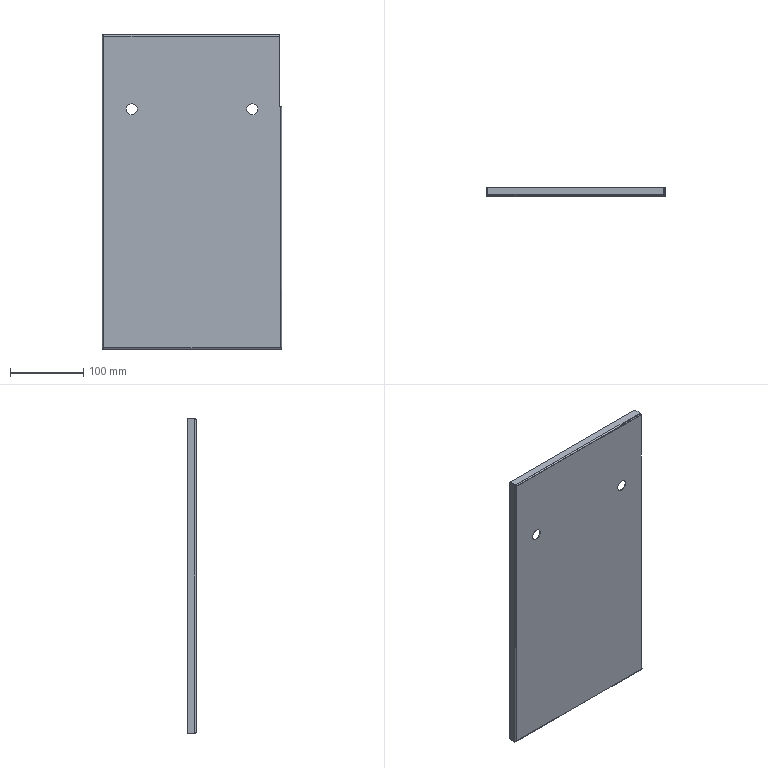Part | 1 solid | 45 faces | box 245 x 12 x 430 mm | volume 140968 mm3 | plane 29 | cylinder 12 | spline 4 | commonest cylinder face diameters 1.48 x4 3.88 x4 15 x4
STEP:
#1=CARTESIAN_POINT('',(75.,0.,113.2));
#2=VERTEX_POINT('',#1);
#3=CARTESIAN_POINT('',(90.,0.,113.2));
#4=VERTEX_POINT('',#3);
#5=CARTESIAN_POINT('',(82.5,0.,113.2));
#6=DIRECTION('',(0.,-1.,0.));
#7=DIRECTION('',(0.,0.,-1.));
#8=AXIS2_PLACEMENT_3D('',#5,#6,#7);
#9=CIRCLE('',#8,7.5);
#10=EDGE_CURVE('',#2,#4,#9,.T.);
#11=ORIENTED_EDGE('',*,*,#10,.F.);
#12=CARTESIAN_POINT('',(75.,-1.2,113.2));
#13=VERTEX_POINT('',#12);
#14=CARTESIAN_POINT('',(75.,10.8,113.2));
#15=DIRECTION('',(0.,-1.,0.));
#16=VECTOR('',#15,1000.);
#17=LINE('',#14,#16);
#18=EDGE_CURVE('',#2,#13,#17,.T.);
#19=ORIENTED_EDGE('',*,*,#18,.T.);
#20=CARTESIAN_POINT('',(90.,-1.2,113.2));
#21=VERTEX_POINT('',#20);
#22=CARTESIAN_POINT('',(82.5,-1.2,113.2));
#23=DIRECTION('',(0.,-1.,0.));
#24=DIRECTION('',(1.,0.,0.));
#25=AXIS2_PLACEMENT_3D('',#22,#23,#24);
#26=CIRCLE('',#25,7.5);
#27=EDGE_CURVE('',#13,#21,#26,.T.);
#28=ORIENTED_EDGE('',*,*,#27,.T.);
#29=CARTESIAN_POINT('',(90.,10.8,113.2));
#30=DIRECTION('',(0.,-1.,0.));
#31=VECTOR('',#30,1000.);
#32=LINE('',#29,#31);
#33=EDGE_CURVE('',#4,#21,#32,.T.);
#34=ORIENTED_EDGE('',*,*,#33,.F.);
#35=EDGE_LOOP('',(#11,#19,#28,#34));
#36=FACE_OUTER_BOUND('',#35,.T.);
#37=CARTESIAN_POINT('',(82.5,10.8,113.2));
#38=DIRECTION('',(0.,-1.,0.));
#39=DIRECTION('',(1.,0.,0.));
#40=AXIS2_PLACEMENT_3D('',#37,#38,#39);
#41=CYLINDRICAL_SURFACE('',#40,7.5);
#42=ADVANCED_FACE('',(#36),#41,.F.);
#43=CARTESIAN_POINT('',(-90.,0.,113.2));
#44=VERTEX_POINT('',#43);
#45=CARTESIAN_POINT('',(-75.,0.,113.2));
#46=VERTEX_POINT('',#45);
#47=CARTESIAN_POINT('',(-82.5,0.,113.2));
#48=DIRECTION('',(0.,-1.,0.));
#49=DIRECTION('',(0.,0.,-1.));
#50=AXIS2_PLACEMENT_3D('',#47,#48,#49);
#51=CIRCLE('',#50,7.5);
#52=EDGE_CURVE('',#44,#46,#51,.T.);
#53=ORIENTED_EDGE('',*,*,#52,.F.);
#54=CARTESIAN_POINT('',(-90.,-1.2,113.2));
#55=VERTEX_POINT('',#54);
#56=CARTESIAN_POINT('',(-90.,10.8,113.2));
#57=DIRECTION('',(0.,-1.,0.));
#58=VECTOR('',#57,1000.);
#59=LINE('',#56,#58);
#60=EDGE_CURVE('',#44,#55,#59,.T.);
#61=ORIENTED_EDGE('',*,*,#60,.T.);
#62=CARTESIAN_POINT('',(-75.,-1.2,113.2));
#63=VERTEX_POINT('',#62);
#64=CARTESIAN_POINT('',(-82.5,-1.2,113.2));
#65=DIRECTION('',(0.,-1.,0.));
#66=DIRECTION('',(1.,0.,0.));
#67=AXIS2_PLACEMENT_3D('',#64,#65,#66);
#68=CIRCLE('',#67,7.5);
#69=EDGE_CURVE('',#55,#63,#68,.T.);
#70=ORIENTED_EDGE('',*,*,#69,.T.);
#71=CARTESIAN_POINT('',(-75.,10.8,113.2));
#72=DIRECTION('',(0.,-1.,0.));
#73=VECTOR('',#72,1000.);
#74=LINE('',#71,#73);
#75=EDGE_CURVE('',#46,#63,#74,.T.);
#76=ORIENTED_EDGE('',*,*,#75,.F.);
#77=EDGE_LOOP('',(#53,#61,#70,#76));
#78=FACE_OUTER_BOUND('',#77,.T.);
#79=CARTESIAN_POINT('',(-82.5,10.8,113.2));
#80=DIRECTION('',(0.,-1.,0.));
#81=DIRECTION('',(1.,0.,0.));
#82=AXIS2_PLACEMENT_3D('',#79,#80,#81);
#83=CYLINDRICAL_SURFACE('',#82,7.5);
#84=ADVANCED_FACE('',(#78),#83,.F.);
#85=CARTESIAN_POINT('',(82.5,-1.2,113.2));
#86=DIRECTION('',(0.,-1.,0.));
#87=DIRECTION('',(1.,0.,0.));
#88=AXIS2_PLACEMENT_3D('',#85,#86,#87);
#89=CIRCLE('',#88,7.5);
#90=EDGE_CURVE('',#21,#13,#89,.T.);
#91=ORIENTED_EDGE('',*,*,#90,.F.);
#92=ORIENTED_EDGE('',*,*,#27,.F.);
#93=EDGE_LOOP('',(#91,#92));
#94=FACE_BOUND('',#93,.T.);
#95=CARTESIAN_POINT('',(-82.5,-1.2,113.2));
#96=DIRECTION('',(0.,-1.,0.));
#97=DIRECTION('',(1.,0.,0.));
#98=AXIS2_PLACEMENT_3D('',#95,#96,#97);
#99=CIRCLE('',#98,7.5);
#100=EDGE_CURVE('',#63,#55,#99,.T.);
#101=ORIENTED_EDGE('',*,*,#100,.F.);
#102=ORIENTED_EDGE('',*,*,#69,.F.);
#103=EDGE_LOOP('',(#101,#102));
#104=FACE_BOUND('',#103,.T.);
#105=CARTESIAN_POINT('',(119.96,-1.2,116.94));
#106=VERTEX_POINT('',#105);
#107=CARTESIAN_POINT('',(119.96,-1.2,213.06));
#108=VERTEX_POINT('',#107);
#109=CARTESIAN_POINT('',(119.96,-1.2,0.));
#110=DIRECTION('',(0.,0.,1.));
#111=VECTOR('',#110,1000.);
#112=LINE('',#109,#111);
#113=EDGE_CURVE('',#106,#108,#112,.T.);
#114=ORIENTED_EDGE('',*,*,#113,.T.);
#115=CARTESIAN_POINT('',(-120.56,-1.2,213.06));
#116=VERTEX_POINT('',#115);
#117=CARTESIAN_POINT('',(122.5,-1.2,213.06));
#118=DIRECTION('',(-1.,0.,0.));
#119=VECTOR('',#118,1000.);
#120=LINE('',#117,#119);
#121=EDGE_CURVE('',#108,#116,#120,.T.);
#122=ORIENTED_EDGE('',*,*,#121,.T.);
#123=CARTESIAN_POINT('',(-120.56,-1.2,-213.06));
#124=VERTEX_POINT('',#123);
#125=CARTESIAN_POINT('',(-120.56,-1.2,213.446));
#126=DIRECTION('',(0.,0.,-1.));
#127=VECTOR('',#126,1000.);
#128=LINE('',#125,#127);
#129=EDGE_CURVE('',#116,#124,#128,.T.);
#130=ORIENTED_EDGE('',*,*,#129,.T.);
#131=CARTESIAN_POINT('',(120.56,-1.2,-213.06));
#132=VERTEX_POINT('',#131);
#133=CARTESIAN_POINT('',(-120.946,-1.2,-213.06));
#134=DIRECTION('',(1.,0.,0.));
#135=VECTOR('',#134,1000.);
#136=LINE('',#133,#135);
#137=EDGE_CURVE('',#124,#132,#136,.T.);
#138=ORIENTED_EDGE('',*,*,#137,.T.);
#139=CARTESIAN_POINT('',(120.56,-1.2,116.94));
#140=VERTEX_POINT('',#139);
#141=CARTESIAN_POINT('',(120.56,-1.2,-213.06));
#142=DIRECTION('',(0.,0.,1.));
#143=VECTOR('',#142,1000.);
#144=LINE('',#141,#143);
#145=EDGE_CURVE('',#132,#140,#144,.T.);
#146=ORIENTED_EDGE('',*,*,#145,.T.);
#147=CARTESIAN_POINT('',(0.,-1.2,116.94));
#148=DIRECTION('',(-1.,0.,0.));
#149=VECTOR('',#148,1000.);
#150=LINE('',#147,#149);
#151=EDGE_CURVE('',#140,#106,#150,.T.);
#152=ORIENTED_EDGE('',*,*,#151,.T.);
#153=EDGE_LOOP('',(#114,#122,#130,#138,#146,#152));
#154=FACE_OUTER_BOUND('',#153,.T.);
#155=CARTESIAN_POINT('',(0.,-1.2,0.));
#156=DIRECTION('',(0.,-1.,0.));
#157=DIRECTION('',(0.,0.,-1.));
#158=AXIS2_PLACEMENT_3D('',#155,#156,#157);
#159=PLANE('',#158);
#160=ADVANCED_FACE('',(#94,#104,#154),#159,.T.);
#161=CARTESIAN_POINT('',(82.5,0.,113.2));
#162=DIRECTION('',(0.,-1.,0.));
#163=DIRECTION('',(0.,0.,-1.));
#164=AXIS2_PLACEMENT_3D('',#161,#162,#163);
#165=CIRCLE('',#164,7.5);
#166=EDGE_CURVE('',#4,#2,#165,.T.);
#167=ORIENTED_EDGE('',*,*,#166,.T.);
#168=ORIENTED_EDGE('',*,*,#10,.T.);
#169=EDGE_LOOP('',(#167,#168));
#170=FACE_BOUND('',#169,.T.);
#171=CARTESIAN_POINT('',(-82.5,0.,113.2));
#172=DIRECTION('',(0.,-1.,0.));
#173=DIRECTION('',(0.,0.,-1.));
#174=AXIS2_PLACEMENT_3D('',#171,#172,#173);
#175=CIRCLE('',#174,7.5);
#176=EDGE_CURVE('',#46,#44,#175,.T.);
#177=ORIENTED_EDGE('',*,*,#176,.T.);
#178=ORIENTED_EDGE('',*,*,#52,.T.);
#179=EDGE_LOOP('',(#177,#178));
#180=FACE_BOUND('',#179,.T.);
#181=CARTESIAN_POINT('',(119.96,0.,213.06));
#182=VERTEX_POINT('',#181);
#183=CARTESIAN_POINT('',(-120.56,0.,213.06));
#184=VERTEX_POINT('',#183);
#185=CARTESIAN_POINT('',(122.5,0.,213.06));
#186=DIRECTION('',(-1.,0.,0.));
#187=VECTOR('',#186,1000.);
#188=LINE('',#185,#187);
#189=EDGE_CURVE('',#182,#184,#188,.T.);
#190=ORIENTED_EDGE('',*,*,#189,.F.);
#191=CARTESIAN_POINT('',(119.96,0.,116.94));
#192=VERTEX_POINT('',#191);
#193=CARTESIAN_POINT('',(119.96,0.,116.94));
#194=DIRECTION('',(0.,0.,1.));
#195=VECTOR('',#194,1000.);
#196=LINE('',#193,#195);
#197=EDGE_CURVE('',#192,#182,#196,.T.);
#198=ORIENTED_EDGE('',*,*,#197,.F.);
#199=CARTESIAN_POINT('',(120.56,0.,116.94));
#200=VERTEX_POINT('',#199);
#201=CARTESIAN_POINT('',(120.56,0.,116.94));
#202=DIRECTION('',(-1.,0.,0.));
#203=VECTOR('',#202,1000.);
#204=LINE('',#201,#203);
#205=EDGE_CURVE('',#200,#192,#204,.T.);
#206=ORIENTED_EDGE('',*,*,#205,.F.);
#207=CARTESIAN_POINT('',(120.56,0.,-213.06));
#208=VERTEX_POINT('',#207);
#209=CARTESIAN_POINT('',(120.56,0.,-213.06));
#210=DIRECTION('',(0.,0.,1.));
#211=VECTOR('',#210,1000.);
#212=LINE('',#209,#211);
#213=EDGE_CURVE('',#208,#200,#212,.T.);
#214=ORIENTED_EDGE('',*,*,#213,.F.);
#215=CARTESIAN_POINT('',(-120.56,0.,-213.06));
#216=VERTEX_POINT('',#215);
#217=CARTESIAN_POINT('',(-120.946,0.,-213.06));
#218=DIRECTION('',(1.,0.,0.));
#219=VECTOR('',#218,1000.);
#220=LINE('',#217,#219);
#221=EDGE_CURVE('',#216,#208,#220,.T.);
#222=ORIENTED_EDGE('',*,*,#221,.F.);
#223=CARTESIAN_POINT('',(-120.56,0.,213.446));
#224=DIRECTION('',(0.,0.,-1.));
#225=VECTOR('',#224,1000.);
#226=LINE('',#223,#225);
#227=EDGE_CURVE('',#184,#216,#226,.T.);
#228=ORIENTED_EDGE('',*,*,#227,.F.);
#229=EDGE_LOOP('',(#190,#198,#206,#214,#222,#228));
#230=FACE_OUTER_BOUND('',#229,.T.);
#231=CARTESIAN_POINT('',(0.,0.,0.));
#232=DIRECTION('',(0.,-1.,0.));
#233=DIRECTION('',(0.,0.,-1.));
#234=AXIS2_PLACEMENT_3D('',#231,#232,#233);
#235=PLANE('',#234);
#236=ADVANCED_FACE('',(#170,#180,#230),#235,.F.);
#237=ORIENTED_EDGE('',*,*,#121,.F.);
#238=CARTESIAN_POINT('',(119.96,0.74,215.));
#239=VERTEX_POINT('',#238);
#240=CARTESIAN_POINT('',(119.96,0.74,213.06));
#241=DIRECTION('',(-1.,0.,0.));
#242=DIRECTION('',(0.,0.,1.));
#243=AXIS2_PLACEMENT_3D('',#240,#241,#242);
#244=CIRCLE('',#243,1.94);
#245=EDGE_CURVE('',#108,#239,#244,.T.);
#246=ORIENTED_EDGE('',*,*,#245,.T.);
#247=CARTESIAN_POINT('',(-121.2,0.74,215.));
#248=VERTEX_POINT('',#247);
#249=CARTESIAN_POINT('',(-122.5,0.74,215.));
#250=DIRECTION('',(-1.,0.,0.));
#251=VECTOR('',#250,1000.);
#252=LINE('',#249,#251);
#253=EDGE_CURVE('',#239,#248,#252,.T.);
#254=ORIENTED_EDGE('',*,*,#253,.T.);
#255=CARTESIAN_POINT('',(-121.2,0.74,215.));
#256=CARTESIAN_POINT('',(-121.173,0.612,215.));
#257=CARTESIAN_POINT('',(-121.147,0.4858,214.987));
#258=CARTESIAN_POINT('',(-121.093,0.2373,214.938));
#259=CARTESIAN_POINT('',(-121.066,0.1139,214.901));
#260=CARTESIAN_POINT('',(-121.013,-0.1202,214.803));
#261=CARTESIAN_POINT('',(-120.987,-0.2316,214.744));
#262=CARTESIAN_POINT('',(-120.934,-0.4427,214.603));
#263=CARTESIAN_POINT('',(-120.907,-0.5422,214.521));
#264=CARTESIAN_POINT('',(-120.827,-0.8103,214.253));
#265=CARTESIAN_POINT('',(-120.773,-0.9549,214.037));
#266=CARTESIAN_POINT('',(-120.667,-1.149,213.571));
#267=CARTESIAN_POINT('',(-120.614,-1.2,213.316));
#268=CARTESIAN_POINT('',(-120.56,-1.2,213.06));
#269=B_SPLINE_CURVE_WITH_KNOTS('',3,(#255,#256,#257,#258,#259,#260,#261,#262,#263,#264,#265,#266,#267,#268),.UNSPECIFIED.,.F.,.F.,(4,2,2,2,2,2,4),(0.,0.000388,0.000776,0.001164,0.001552,0.002328,0.003104),.UNSPECIFIED.);
#270=EDGE_CURVE('',#248,#116,#269,.T.);
#271=ORIENTED_EDGE('',*,*,#270,.T.);
#272=EDGE_LOOP('',(#237,#246,#254,#271));
#273=FACE_OUTER_BOUND('',#272,.T.);
#274=CARTESIAN_POINT('',(244.68,0.74,213.06));
#275=DIRECTION('',(-1.,0.,0.));
#276=DIRECTION('',(0.,0.,1.));
#277=AXIS2_PLACEMENT_3D('',#274,#275,#276);
#278=CYLINDRICAL_SURFACE('',#277,1.94);
#279=ADVANCED_FACE('',(#273),#278,.T.);
#280=CARTESIAN_POINT('',(119.96,0.74,213.8));
#281=VERTEX_POINT('',#280);
#282=CARTESIAN_POINT('',(119.96,0.74,213.06));
#283=DIRECTION('',(-1.,0.,0.));
#284=DIRECTION('',(0.,0.,1.));
#285=AXIS2_PLACEMENT_3D('',#282,#283,#284);
#286=CIRCLE('',#285,0.74);
#287=EDGE_CURVE('',#182,#281,#286,.T.);
#288=ORIENTED_EDGE('',*,*,#287,.F.);
#289=ORIENTED_EDGE('',*,*,#189,.T.);
#290=CARTESIAN_POINT('',(-121.2,0.74,213.8));
#291=VERTEX_POINT('',#290);
#292=CARTESIAN_POINT('',(-121.2,0.74,213.8));
#293=CARTESIAN_POINT('',(-121.093,0.5463,213.8));
#294=CARTESIAN_POINT('',(-120.987,0.3537,213.72));
#295=CARTESIAN_POINT('',(-120.773,0.07975,213.446));
#296=CARTESIAN_POINT('',(-120.667,0.,213.254));
#297=CARTESIAN_POINT('',(-120.56,0.,213.06));
#298=B_SPLINE_CURVE_WITH_KNOTS('',3,(#292,#293,#294,#295,#296,#297),.UNSPECIFIED.,.F.,.F.,(4,2,4),(0.,0.5,1.),.UNSPECIFIED.);
#299=EDGE_CURVE('',#291,#184,#298,.T.);
#300=ORIENTED_EDGE('',*,*,#299,.F.);
#301=CARTESIAN_POINT('',(-122.5,0.74,213.8));
#302=DIRECTION('',(1.,0.,0.));
#303=VECTOR('',#302,1000.);
#304=LINE('',#301,#303);
#305=EDGE_CURVE('',#291,#281,#304,.T.);
#306=ORIENTED_EDGE('',*,*,#305,.T.);
#307=EDGE_LOOP('',(#288,#289,#300,#306));
#308=FACE_OUTER_BOUND('',#307,.T.);
#309=CARTESIAN_POINT('',(244.68,0.74,213.06));
#310=DIRECTION('',(-1.,0.,0.));
#311=DIRECTION('',(0.,0.,1.));
#312=AXIS2_PLACEMENT_3D('',#309,#310,#311);
#313=CYLINDRICAL_SURFACE('',#312,0.74);
#314=ADVANCED_FACE('',(#308),#313,.F.);
#315=CARTESIAN_POINT('',(-121.2,10.8,215.));
#316=VERTEX_POINT('',#315);
#317=CARTESIAN_POINT('',(119.96,10.8,215.));
#318=VERTEX_POINT('',#317);
#319=CARTESIAN_POINT('',(-122.5,10.8,215.));
#320=DIRECTION('',(1.,0.,0.));
#321=VECTOR('',#320,1000.);
#322=LINE('',#319,#321);
#323=EDGE_CURVE('',#316,#318,#322,.T.);
#324=ORIENTED_EDGE('',*,*,#323,.T.);
#325=CARTESIAN_POINT('',(119.96,10.8,213.8));
#326=VERTEX_POINT('',#325);
#327=CARTESIAN_POINT('',(119.96,10.8,213.8));
#328=DIRECTION('',(0.,0.,-1.));
#329=VECTOR('',#328,1000.);
#330=LINE('',#327,#329);
#331=EDGE_CURVE('',#318,#326,#330,.T.);
#332=ORIENTED_EDGE('',*,*,#331,.T.);
#333=CARTESIAN_POINT('',(-121.2,10.8,213.8));
#334=VERTEX_POINT('',#333);
#335=CARTESIAN_POINT('',(0.,10.8,213.8));
#336=DIRECTION('',(1.,0.,0.));
#337=VECTOR('',#336,1000.);
#338=LINE('',#335,#337);
#339=EDGE_CURVE('',#334,#326,#338,.T.);
#340=ORIENTED_EDGE('',*,*,#339,.F.);
#341=CARTESIAN_POINT('',(-121.2,10.8,213.8));
#342=DIRECTION('',(0.,0.,1.));
#343=VECTOR('',#342,1000.);
#344=LINE('',#341,#343);
#345=EDGE_CURVE('',#334,#316,#344,.T.);
#346=ORIENTED_EDGE('',*,*,#345,.T.);
#347=EDGE_LOOP('',(#324,#332,#340,#346));
#348=FACE_OUTER_BOUND('',#347,.T.);
#349=CARTESIAN_POINT('',(-122.5,10.8,215.));
#350=DIRECTION('',(0.,1.,0.));
#351=DIRECTION('',(0.,0.,1.));
#352=AXIS2_PLACEMENT_3D('',#349,#350,#351);
#353=PLANE('',#352);
#354=ADVANCED_FACE('',(#348),#353,.T.);
#355=CARTESIAN_POINT('',(119.96,5.77,215.));
#356=DIRECTION('',(0.,-1.,0.));
#357=VECTOR('',#356,1000.);
#358=LINE('',#355,#357);
#359=EDGE_CURVE('',#318,#239,#358,.T.);
#360=ORIENTED_EDGE('',*,*,#359,.F.);
#361=ORIENTED_EDGE('',*,*,#323,.F.);
#362=CARTESIAN_POINT('',(-121.2,0.74,215.));
#363=DIRECTION('',(0.,1.,0.));
#364=VECTOR('',#363,1000.);
#365=LINE('',#362,#364);
#366=EDGE_CURVE('',#248,#316,#365,.T.);
#367=ORIENTED_EDGE('',*,*,#366,.F.);
#368=ORIENTED_EDGE('',*,*,#253,.F.);
#369=EDGE_LOOP('',(#360,#361,#367,#368));
#370=FACE_OUTER_BOUND('',#369,.T.);
#371=CARTESIAN_POINT('',(0.,0.,215.));
#372=DIRECTION('',(0.,0.,-1.));
#373=DIRECTION('',(0.,1.,0.));
#374=AXIS2_PLACEMENT_3D('',#371,#372,#373);
#375=PLANE('',#374);
#376=ADVANCED_FACE('',(#370),#375,.F.);
#377=ORIENTED_EDGE('',*,*,#339,.T.);
#378=CARTESIAN_POINT('',(119.96,10.8,213.8));
#379=DIRECTION('',(0.,-1.,0.));
#380=VECTOR('',#379,1000.);
#381=LINE('',#378,#380);
#382=EDGE_CURVE('',#326,#281,#381,.T.);
#383=ORIENTED_EDGE('',*,*,#382,.T.);
#384=ORIENTED_EDGE('',*,*,#305,.F.);
#385=CARTESIAN_POINT('',(-121.2,0.74,213.8));
#386=DIRECTION('',(0.,1.,0.));
#387=VECTOR('',#386,1000.);
#388=LINE('',#385,#387);
#389=EDGE_CURVE('',#291,#334,#388,.T.);
#390=ORIENTED_EDGE('',*,*,#389,.T.);
#391=EDGE_LOOP('',(#377,#383,#384,#390));
#392=FACE_OUTER_BOUND('',#391,.T.);
#393=CARTESIAN_POINT('',(0.,0.,213.8));
#394=DIRECTION('',(0.,0.,-1.));
#395=DIRECTION('',(0.,1.,0.));
#396=AXIS2_PLACEMENT_3D('',#393,#394,#395);
#397=PLANE('',#396);
#398=ADVANCED_FACE('',(#392),#397,.T.);
#399=ORIENTED_EDGE('',*,*,#60,.F.);
#400=ORIENTED_EDGE('',*,*,#176,.F.);
#401=ORIENTED_EDGE('',*,*,#75,.T.);
#402=ORIENTED_EDGE('',*,*,#100,.T.);
#403=EDGE_LOOP('',(#399,#400,#401,#402));
#404=FACE_OUTER_BOUND('',#403,.T.);
#405=CARTESIAN_POINT('',(-82.5,10.8,113.2));
#406=DIRECTION('',(0.,-1.,0.));
#407=DIRECTION('',(1.,0.,0.));
#408=AXIS2_PLACEMENT_3D('',#405,#406,#407);
#409=CYLINDRICAL_SURFACE('',#408,7.5);
#410=ADVANCED_FACE('',(#404),#409,.F.);
#411=ORIENTED_EDGE('',*,*,#18,.F.);
#412=ORIENTED_EDGE('',*,*,#166,.F.);
#413=ORIENTED_EDGE('',*,*,#33,.T.);
#414=ORIENTED_EDGE('',*,*,#90,.T.);
#415=EDGE_LOOP('',(#411,#412,#413,#414));
#416=FACE_OUTER_BOUND('',#415,.T.);
#417=CARTESIAN_POINT('',(82.5,10.8,113.2));
#418=DIRECTION('',(0.,-1.,0.));
#419=DIRECTION('',(1.,0.,0.));
#420=AXIS2_PLACEMENT_3D('',#417,#418,#419);
#421=CYLINDRICAL_SURFACE('',#420,7.5);
#422=ADVANCED_FACE('',(#416),#421,.F.);
#423=ORIENTED_EDGE('',*,*,#151,.F.);
#424=CARTESIAN_POINT('',(120.56,0.,116.94));
#425=DIRECTION('',(0.,-1.,0.));
#426=VECTOR('',#425,1000.);
#427=LINE('',#424,#426);
#428=EDGE_CURVE('',#200,#140,#427,.T.);
#429=ORIENTED_EDGE('',*,*,#428,.F.);
#430=ORIENTED_EDGE('',*,*,#205,.T.);
#431=CARTESIAN_POINT('',(119.96,0.,116.94));
#432=DIRECTION('',(0.,-1.,0.));
#433=VECTOR('',#432,1000.);
#434=LINE('',#431,#433);
#435=EDGE_CURVE('',#192,#106,#434,.T.);
#436=ORIENTED_EDGE('',*,*,#435,.T.);
#437=EDGE_LOOP('',(#423,#429,#430,#436));
#438=FACE_OUTER_BOUND('',#437,.T.);
#439=CARTESIAN_POINT('',(120.56,0.,116.94));
#440=DIRECTION('',(0.,0.,1.));
#441=DIRECTION('',(0.,-1.,0.));
#442=AXIS2_PLACEMENT_3D('',#439,#440,#441);
#443=PLANE('',#442);
#444=ADVANCED_FACE('',(#438),#443,.T.);
#445=ORIENTED_EDGE('',*,*,#113,.F.);
#446=ORIENTED_EDGE('',*,*,#435,.F.);
#447=ORIENTED_EDGE('',*,*,#197,.T.);
#448=CARTESIAN_POINT('',(119.96,-1.2,213.06));
#449=DIRECTION('',(0.,1.,0.));
#450=VECTOR('',#449,1000.);
#451=LINE('',#448,#450);
#452=EDGE_CURVE('',#108,#182,#451,.T.);
#453=ORIENTED_EDGE('',*,*,#452,.F.);
#454=EDGE_LOOP('',(#445,#446,#447,#453));
#455=FACE_OUTER_BOUND('',#454,.T.);
#456=CARTESIAN_POINT('',(119.96,0.,116.94));
#457=DIRECTION('',(1.,0.,0.));
#458=DIRECTION('',(0.,0.,-1.));
#459=AXIS2_PLACEMENT_3D('',#456,#457,#458);
#460=PLANE('',#459);
#461=ADVANCED_FACE('',(#455),#460,.T.);
#462=CARTESIAN_POINT('',(121.3,0.74,116.94));
#463=VERTEX_POINT('',#462);
#464=CARTESIAN_POINT('',(122.5,0.74,116.94));
#465=VERTEX_POINT('',#464);
#466=CARTESIAN_POINT('',(122.5,0.74,116.94));
#467=DIRECTION('',(1.,0.,0.));
#468=VECTOR('',#467,1000.);
#469=LINE('',#466,#468);
#470=EDGE_CURVE('',#463,#465,#469,.T.);
#471=ORIENTED_EDGE('',*,*,#470,.F.);
#472=CARTESIAN_POINT('',(120.56,0.74,116.94));
#473=DIRECTION('',(0.,0.,1.));
#474=DIRECTION('',(0.,1.,0.));
#475=AXIS2_PLACEMENT_3D('',#472,#473,#474);
#476=CIRCLE('',#475,0.74);
#477=EDGE_CURVE('',#200,#463,#476,.T.);
#478=ORIENTED_EDGE('',*,*,#477,.F.);
#479=ORIENTED_EDGE('',*,*,#428,.T.);
#480=CARTESIAN_POINT('',(120.56,0.74,116.94));
#481=DIRECTION('',(0.,0.,1.));
#482=DIRECTION('',(0.,1.,0.));
#483=AXIS2_PLACEMENT_3D('',#480,#481,#482);
#484=CIRCLE('',#483,1.94);
#485=EDGE_CURVE('',#140,#465,#484,.T.);
#486=ORIENTED_EDGE('',*,*,#485,.T.);
#487=EDGE_LOOP('',(#471,#478,#479,#486));
#488=FACE_OUTER_BOUND('',#487,.T.);
#489=CARTESIAN_POINT('',(120.56,0.74,116.94));
#490=DIRECTION('',(0.,0.,1.));
#491=DIRECTION('',(0.,-1.,0.));
#492=AXIS2_PLACEMENT_3D('',#489,#490,#491);
#493=PLANE('',#492);
#494=ADVANCED_FACE('',(#488),#493,.T.);
#495=CARTESIAN_POINT('',(122.5,0.74,-213.06));
#496=VERTEX_POINT('',#495);
#497=CARTESIAN_POINT('',(122.353,0.,-213.06));
#498=VERTEX_POINT('',#497);
#499=CARTESIAN_POINT('',(120.56,0.74,-213.06));
#500=DIRECTION('',(0.,0.,-1.));
#501=DIRECTION('',(0.,1.,0.));
#502=AXIS2_PLACEMENT_3D('',#499,#500,#501);
#503=CIRCLE('',#502,1.94);
#504=EDGE_CURVE('',#496,#498,#503,.T.);
#505=ORIENTED_EDGE('',*,*,#504,.T.);
#506=CARTESIAN_POINT('',(122.5,0.,-213.06));
#507=DIRECTION('',(-1.,0.,0.));
#508=VECTOR('',#507,1000.);
#509=LINE('',#506,#508);
#510=EDGE_CURVE('',#498,#208,#509,.T.);
#511=ORIENTED_EDGE('',*,*,#510,.T.);
#512=CARTESIAN_POINT('',(121.3,0.74,-213.06));
#513=VERTEX_POINT('',#512);
#514=CARTESIAN_POINT('',(120.56,0.74,-213.06));
#515=DIRECTION('',(0.,0.,-1.));
#516=DIRECTION('',(0.,1.,0.));
#517=AXIS2_PLACEMENT_3D('',#514,#515,#516);
#518=CIRCLE('',#517,0.74);
#519=EDGE_CURVE('',#513,#208,#518,.T.);
#520=ORIENTED_EDGE('',*,*,#519,.F.);
#521=CARTESIAN_POINT('',(121.3,0.74,-213.06));
#522=DIRECTION('',(1.,0.,0.));
#523=VECTOR('',#522,1000.);
#524=LINE('',#521,#523);
#525=EDGE_CURVE('',#513,#496,#524,.T.);
#526=ORIENTED_EDGE('',*,*,#525,.T.);
#527=EDGE_LOOP('',(#505,#511,#520,#526));
#528=FACE_OUTER_BOUND('',#527,.T.);
#529=CARTESIAN_POINT('',(120.56,0.74,-213.06));
#530=DIRECTION('',(0.,0.,1.));
#531=DIRECTION('',(0.,-1.,0.));
#532=AXIS2_PLACEMENT_3D('',#529,#530,#531);
#533=PLANE('',#532);
#534=ADVANCED_FACE('',(#528),#533,.F.);
#535=ORIENTED_EDGE('',*,*,#145,.F.);
#536=CARTESIAN_POINT('',(120.56,0.74,-213.06));
#537=DIRECTION('',(0.,0.,-1.));
#538=DIRECTION('',(0.,1.,0.));
#539=AXIS2_PLACEMENT_3D('',#536,#537,#538);
#540=CIRCLE('',#539,1.94);
#541=EDGE_CURVE('',#498,#132,#540,.T.);
#542=ORIENTED_EDGE('',*,*,#541,.F.);
#543=ORIENTED_EDGE('',*,*,#504,.F.);
#544=CARTESIAN_POINT('',(122.5,0.74,0.));
#545=DIRECTION('',(0.,0.,-1.));
#546=VECTOR('',#545,1000.);
#547=LINE('',#544,#546);
#548=EDGE_CURVE('',#465,#496,#547,.T.);
#549=ORIENTED_EDGE('',*,*,#548,.F.);
#550=ORIENTED_EDGE('',*,*,#485,.F.);
#551=EDGE_LOOP('',(#535,#542,#543,#549,#550));
#552=FACE_OUTER_BOUND('',#551,.T.);
#553=CARTESIAN_POINT('',(120.56,0.74,-213.06));
#554=DIRECTION('',(0.,0.,-1.));
#555=DIRECTION('',(1.,0.,0.));
#556=AXIS2_PLACEMENT_3D('',#553,#554,#555);
#557=CYLINDRICAL_SURFACE('',#556,1.94);
#558=ADVANCED_FACE('',(#552),#557,.T.);
#559=ORIENTED_EDGE('',*,*,#213,.T.);
#560=ORIENTED_EDGE('',*,*,#477,.T.);
#561=CARTESIAN_POINT('',(121.3,0.74,116.94));
#562=DIRECTION('',(0.,0.,-1.));
#563=VECTOR('',#562,1000.);
#564=LINE('',#561,#563);
#565=EDGE_CURVE('',#463,#513,#564,.T.);
#566=ORIENTED_EDGE('',*,*,#565,.T.);
#567=ORIENTED_EDGE('',*,*,#519,.T.);
#568=EDGE_LOOP('',(#559,#560,#566,#567));
#569=FACE_OUTER_BOUND('',#568,.T.);
#570=CARTESIAN_POINT('',(120.56,0.74,-213.06));
#571=DIRECTION('',(0.,0.,-1.));
#572=DIRECTION('',(1.,0.,0.));
#573=AXIS2_PLACEMENT_3D('',#570,#571,#572);
#574=CYLINDRICAL_SURFACE('',#573,0.74);
#575=ADVANCED_FACE('',(#569),#574,.F.);
#576=CARTESIAN_POINT('',(122.5,10.8,-213.06));
#577=VERTEX_POINT('',#576);
#578=CARTESIAN_POINT('',(122.5,0.,-213.06));
#579=DIRECTION('',(0.,-1.,0.));
#580=VECTOR('',#579,1000.);
#581=LINE('',#578,#580);
#582=EDGE_CURVE('',#577,#496,#581,.T.);
#583=ORIENTED_EDGE('',*,*,#582,.T.);
#584=ORIENTED_EDGE('',*,*,#525,.F.);
#585=CARTESIAN_POINT('',(121.3,10.8,-213.06));
#586=VERTEX_POINT('',#585);
#587=CARTESIAN_POINT('',(121.3,0.,-213.06));
#588=DIRECTION('',(0.,-1.,0.));
#589=VECTOR('',#588,1000.);
#590=LINE('',#587,#589);
#591=EDGE_CURVE('',#586,#513,#590,.T.);
#592=ORIENTED_EDGE('',*,*,#591,.F.);
#593=CARTESIAN_POINT('',(122.5,10.8,-213.06));
#594=DIRECTION('',(-1.,0.,0.));
#595=VECTOR('',#594,1000.);
#596=LINE('',#593,#595);
#597=EDGE_CURVE('',#577,#586,#596,.T.);
#598=ORIENTED_EDGE('',*,*,#597,.F.);
#599=EDGE_LOOP('',(#583,#584,#592,#598));
#600=FACE_OUTER_BOUND('',#599,.T.);
#601=CARTESIAN_POINT('',(122.5,0.,-213.06));
#602=DIRECTION('',(0.,0.,-1.));
#603=DIRECTION('',(0.,1.,0.));
#604=AXIS2_PLACEMENT_3D('',#601,#602,#603);
#605=PLANE('',#604);
#606=ADVANCED_FACE('',(#600),#605,.T.);
#607=CARTESIAN_POINT('',(121.3,10.8,116.94));
#608=VERTEX_POINT('',#607);
#609=CARTESIAN_POINT('',(121.3,0.,116.94));
#610=DIRECTION('',(0.,1.,0.));
#611=VECTOR('',#610,1000.);
#612=LINE('',#609,#611);
#613=EDGE_CURVE('',#463,#608,#612,.T.);
#614=ORIENTED_EDGE('',*,*,#613,.F.);
#615=ORIENTED_EDGE('',*,*,#470,.T.);
#616=CARTESIAN_POINT('',(122.5,10.8,116.94));
#617=VERTEX_POINT('',#616);
#618=CARTESIAN_POINT('',(122.5,10.8,116.94));
#619=DIRECTION('',(0.,1.,0.));
#620=VECTOR('',#619,1000.);
#621=LINE('',#618,#620);
#622=EDGE_CURVE('',#465,#617,#621,.T.);
#623=ORIENTED_EDGE('',*,*,#622,.T.);
#624=CARTESIAN_POINT('',(122.5,10.8,116.94));
#625=DIRECTION('',(-1.,0.,0.));
#626=VECTOR('',#625,1000.);
#627=LINE('',#624,#626);
#628=EDGE_CURVE('',#617,#608,#627,.T.);
#629=ORIENTED_EDGE('',*,*,#628,.T.);
#630=EDGE_LOOP('',(#614,#615,#623,#629));
#631=FACE_OUTER_BOUND('',#630,.T.);
#632=CARTESIAN_POINT('',(122.5,10.8,116.94));
#633=DIRECTION('',(0.,0.,1.));
#634=DIRECTION('',(0.,-1.,0.));
#635=AXIS2_PLACEMENT_3D('',#632,#633,#634);
#636=PLANE('',#635);
#637=ADVANCED_FACE('',(#631),#636,.T.);
#638=ORIENTED_EDGE('',*,*,#622,.F.);
#639=ORIENTED_EDGE('',*,*,#548,.T.);
#640=ORIENTED_EDGE('',*,*,#582,.F.);
#641=CARTESIAN_POINT('',(122.5,10.8,-213.06));
#642=DIRECTION('',(0.,0.,-1.));
#643=VECTOR('',#642,1000.);
#644=LINE('',#641,#643);
#645=EDGE_CURVE('',#617,#577,#644,.T.);
#646=ORIENTED_EDGE('',*,*,#645,.F.);
#647=EDGE_LOOP('',(#638,#639,#640,#646));
#648=FACE_OUTER_BOUND('',#647,.T.);
#649=CARTESIAN_POINT('',(122.5,0.,0.));
#650=DIRECTION('',(1.,0.,0.));
#651=DIRECTION('',(0.,1.,0.));
#652=AXIS2_PLACEMENT_3D('',#649,#650,#651);
#653=PLANE('',#652);
#654=ADVANCED_FACE('',(#648),#653,.T.);
#655=ORIENTED_EDGE('',*,*,#565,.F.);
#656=ORIENTED_EDGE('',*,*,#613,.T.);
#657=CARTESIAN_POINT('',(121.3,10.8,0.));
#658=DIRECTION('',(0.,0.,-1.));
#659=VECTOR('',#658,1000.);
#660=LINE('',#657,#659);
#661=EDGE_CURVE('',#608,#586,#660,.T.);
#662=ORIENTED_EDGE('',*,*,#661,.T.);
#663=ORIENTED_EDGE('',*,*,#591,.T.);
#664=EDGE_LOOP('',(#655,#656,#662,#663));
#665=FACE_OUTER_BOUND('',#664,.T.);
#666=CARTESIAN_POINT('',(121.3,0.,0.));
#667=DIRECTION('',(1.,0.,0.));
#668=DIRECTION('',(0.,1.,0.));
#669=AXIS2_PLACEMENT_3D('',#666,#667,#668);
#670=PLANE('',#669);
#671=ADVANCED_FACE('',(#665),#670,.F.);
#672=ORIENTED_EDGE('',*,*,#661,.F.);
#673=ORIENTED_EDGE('',*,*,#628,.F.);
#674=ORIENTED_EDGE('',*,*,#645,.T.);
#675=ORIENTED_EDGE('',*,*,#597,.T.);
#676=EDGE_LOOP('',(#672,#673,#674,#675));
#677=FACE_OUTER_BOUND('',#676,.T.);
#678=CARTESIAN_POINT('',(122.5,10.8,-213.06));
#679=DIRECTION('',(0.,1.,0.));
#680=DIRECTION('',(-1.,0.,0.));
#681=AXIS2_PLACEMENT_3D('',#678,#679,#680);
#682=PLANE('',#681);
#683=ADVANCED_FACE('',(#677),#682,.T.);
#684=CARTESIAN_POINT('',(-121.2,0.74,213.8));
#685=CARTESIAN_POINT('',(-121.2,0.74,214.2));
#686=CARTESIAN_POINT('',(-121.2,0.74,214.6));
#687=CARTESIAN_POINT('',(-121.2,0.74,215.));
#688=B_SPLINE_CURVE_WITH_KNOTS('',3,(#684,#685,#686,#687),.UNSPECIFIED.,.F.,.F.,(4,4),(0.,1.),.UNSPECIFIED.);
#689=EDGE_CURVE('',#291,#248,#688,.T.);
#690=ORIENTED_EDGE('',*,*,#689,.F.);
#691=ORIENTED_EDGE('',*,*,#299,.T.);
#692=CARTESIAN_POINT('',(-120.56,0.,213.06));
#693=CARTESIAN_POINT('',(-120.56,-1.2,213.06));
#694=B_SPLINE_CURVE_WITH_KNOTS('',1,(#692,#693),.UNSPECIFIED.,.F.,.F.,(2,2),(0.,1.),.UNSPECIFIED.);
#695=EDGE_CURVE('',#184,#116,#694,.T.);
#696=ORIENTED_EDGE('',*,*,#695,.T.);
#697=ORIENTED_EDGE('',*,*,#270,.F.);
#698=EDGE_LOOP('',(#690,#691,#696,#697));
#699=FACE_OUTER_BOUND('',#698,.T.);
#700=CARTESIAN_POINT('',(-121.2,0.74,215.012));
#701=CARTESIAN_POINT('',(-121.147,0.4844,215.012));
#702=CARTESIAN_POINT('',(-121.093,0.2291,214.961));
#703=CARTESIAN_POINT('',(-120.987,-0.2431,214.766));
#704=CARTESIAN_POINT('',(-120.933,-0.4596,214.621));
#705=CARTESIAN_POINT('',(-120.827,-0.8209,214.26));
#706=CARTESIAN_POINT('',(-120.773,-0.9656,214.043));
#707=CARTESIAN_POINT('',(-120.667,-1.161,213.571));
#708=CARTESIAN_POINT('',(-120.613,-1.212,213.316));
#709=CARTESIAN_POINT('',(-120.56,-1.212,213.06));
#710=CARTESIAN_POINT('',(-121.2,0.74,215.));
#711=CARTESIAN_POINT('',(-121.147,0.486,215.));
#712=CARTESIAN_POINT('',(-121.093,0.2322,214.95));
#713=CARTESIAN_POINT('',(-120.987,-0.237,214.755));
#714=CARTESIAN_POINT('',(-120.933,-0.4522,214.611));
#715=CARTESIAN_POINT('',(-120.827,-0.8114,214.252));
#716=CARTESIAN_POINT('',(-120.773,-0.9551,214.037));
#717=CARTESIAN_POINT('',(-120.667,-1.15,213.568));
#718=CARTESIAN_POINT('',(-120.613,-1.2,213.314));
#719=CARTESIAN_POINT('',(-120.56,-1.2,213.06));
#720=CARTESIAN_POINT('',(-121.2,0.74,213.8));
#721=CARTESIAN_POINT('',(-121.147,0.6431,213.8));
#722=CARTESIAN_POINT('',(-121.093,0.5463,213.781));
#723=CARTESIAN_POINT('',(-120.987,0.3673,213.707));
#724=CARTESIAN_POINT('',(-120.933,0.2852,213.652));
#725=CARTESIAN_POINT('',(-120.827,0.1482,213.515));
#726=CARTESIAN_POINT('',(-120.773,0.0934,213.433));
#727=CARTESIAN_POINT('',(-120.667,0.01926,213.254));
#728=CARTESIAN_POINT('',(-120.613,0.,213.157));
#729=CARTESIAN_POINT('',(-120.56,0.,213.06));
#730=CARTESIAN_POINT('',(-121.2,0.74,213.788));
#731=CARTESIAN_POINT('',(-121.147,0.6447,213.788));
#732=CARTESIAN_POINT('',(-121.093,0.5495,213.769));
#733=CARTESIAN_POINT('',(-120.987,0.3734,213.696));
#734=CARTESIAN_POINT('',(-120.933,0.2927,213.642));
#735=CARTESIAN_POINT('',(-120.827,0.1579,213.507));
#736=CARTESIAN_POINT('',(-120.773,0.104,213.427));
#737=CARTESIAN_POINT('',(-120.667,0.03106,213.251));
#738=CARTESIAN_POINT('',(-120.613,0.01212,213.155));
#739=CARTESIAN_POINT('',(-120.56,0.01212,213.06));
#740=B_SPLINE_SURFACE_WITH_KNOTS('',1,3,((#700,#701,#702,#703,#704,#705,#706,#707,#708,#709),(#710,#711,#712,#713,#714,#715,#716,#717,#718,#719),(#720,#721,#722,#723,#724,#725,#726,#727,#728,#729),(#730,#731,#732,#733,#734,#735,#736,#737,#738,#739)),.UNSPECIFIED.,.F.,.F.,.F.,(2,1,1,2),(4,2,2,2,4),(-0.01,0.,1.,1.01),(0.,0.25,0.5,0.75,1.),.UNSPECIFIED.);
#741=ADVANCED_FACE('',(#699),#740,.T.);
#742=ORIENTED_EDGE('',*,*,#366,.T.);
#743=ORIENTED_EDGE('',*,*,#345,.F.);
#744=ORIENTED_EDGE('',*,*,#389,.F.);
#745=ORIENTED_EDGE('',*,*,#689,.T.);
#746=EDGE_LOOP('',(#742,#743,#744,#745));
#747=FACE_OUTER_BOUND('',#746,.T.);
#748=CARTESIAN_POINT('',(-121.2,0.74,213.8));
#749=DIRECTION('',(1.,0.,0.));
#750=DIRECTION('',(0.,-1.,0.));
#751=AXIS2_PLACEMENT_3D('',#748,#749,#750);
#752=PLANE('',#751);
#753=ADVANCED_FACE('',(#747),#752,.F.);
#754=CARTESIAN_POINT('',(-122.5,10.8,-215.));
#755=VERTEX_POINT('',#754);
#756=CARTESIAN_POINT('',(-122.5,10.8,215.));
#757=VERTEX_POINT('',#756);
#758=CARTESIAN_POINT('',(-122.5,10.8,-215.));
#759=DIRECTION('',(0.,0.,1.));
#760=VECTOR('',#759,1000.);
#761=LINE('',#758,#760);
#762=EDGE_CURVE('',#755,#757,#761,.T.);
#763=ORIENTED_EDGE('',*,*,#762,.T.);
#764=CARTESIAN_POINT('',(-121.3,10.8,215.));
#765=VERTEX_POINT('',#764);
#766=CARTESIAN_POINT('',(-122.5,10.8,215.));
#767=DIRECTION('',(1.,0.,0.));
#768=VECTOR('',#767,1000.);
#769=LINE('',#766,#768);
#770=EDGE_CURVE('',#757,#765,#769,.T.);
#771=ORIENTED_EDGE('',*,*,#770,.T.);
#772=CARTESIAN_POINT('',(-121.3,10.8,-215.));
#773=VERTEX_POINT('',#772);
#774=CARTESIAN_POINT('',(-121.3,10.8,0.));
#775=DIRECTION('',(0.,0.,1.));
#776=VECTOR('',#775,1000.);
#777=LINE('',#774,#776);
#778=EDGE_CURVE('',#773,#765,#777,.T.);
#779=ORIENTED_EDGE('',*,*,#778,.F.);
#780=CARTESIAN_POINT('',(-122.5,10.8,-215.));
#781=DIRECTION('',(1.,0.,0.));
#782=VECTOR('',#781,1000.);
#783=LINE('',#780,#782);
#784=EDGE_CURVE('',#755,#773,#783,.T.);
#785=ORIENTED_EDGE('',*,*,#784,.F.);
#786=EDGE_LOOP('',(#763,#771,#779,#785));
#787=FACE_OUTER_BOUND('',#786,.T.);
#788=CARTESIAN_POINT('',(-122.5,10.8,-215.));
#789=DIRECTION('',(0.,1.,0.));
#790=DIRECTION('',(-1.,0.,0.));
#791=AXIS2_PLACEMENT_3D('',#788,#789,#790);
#792=PLANE('',#791);
#793=ADVANCED_FACE('',(#787),#792,.T.);
#794=CARTESIAN_POINT('',(-122.5,0.74,215.));
#795=VERTEX_POINT('',#794);
#796=CARTESIAN_POINT('',(-122.5,0.74,-215.));
#797=VERTEX_POINT('',#796);
#798=CARTESIAN_POINT('',(-122.5,0.74,-215.));
#799=DIRECTION('',(0.,0.,-1.));
#800=VECTOR('',#799,1000.);
#801=LINE('',#798,#800);
#802=EDGE_CURVE('',#795,#797,#801,.T.);
#803=ORIENTED_EDGE('',*,*,#802,.F.);
#804=CARTESIAN_POINT('',(-122.5,0.74,215.));
#805=DIRECTION('',(0.,1.,0.));
#806=VECTOR('',#805,1000.);
#807=LINE('',#804,#806);
#808=EDGE_CURVE('',#795,#757,#807,.T.);
#809=ORIENTED_EDGE('',*,*,#808,.T.);
#810=ORIENTED_EDGE('',*,*,#762,.F.);
#811=CARTESIAN_POINT('',(-122.5,0.74,-215.));
#812=DIRECTION('',(0.,1.,0.));
#813=VECTOR('',#812,1000.);
#814=LINE('',#811,#813);
#815=EDGE_CURVE('',#797,#755,#814,.T.);
#816=ORIENTED_EDGE('',*,*,#815,.F.);
#817=EDGE_LOOP('',(#803,#809,#810,#816));
#818=FACE_OUTER_BOUND('',#817,.T.);
#819=CARTESIAN_POINT('',(-122.5,0.,0.));
#820=DIRECTION('',(1.,0.,0.));
#821=DIRECTION('',(0.,1.,0.));
#822=AXIS2_PLACEMENT_3D('',#819,#820,#821);
#823=PLANE('',#822);
#824=ADVANCED_FACE('',(#818),#823,.F.);
#825=CARTESIAN_POINT('',(-121.3,0.74,215.));
#826=VERTEX_POINT('',#825);
#827=CARTESIAN_POINT('',(-121.3,0.74,215.));
#828=DIRECTION('',(0.,1.,0.));
#829=VECTOR('',#828,1000.);
#830=LINE('',#827,#829);
#831=EDGE_CURVE('',#826,#765,#830,.T.);
#832=ORIENTED_EDGE('',*,*,#831,.T.);
#833=ORIENTED_EDGE('',*,*,#770,.F.);
#834=ORIENTED_EDGE('',*,*,#808,.F.);
#835=CARTESIAN_POINT('',(-121.3,0.74,215.));
#836=CARTESIAN_POINT('',(-122.5,0.74,215.));
#837=B_SPLINE_CURVE_WITH_KNOTS('',1,(#835,#836),.UNSPECIFIED.,.F.,.F.,(2,2),(0.,1.),.UNSPECIFIED.);
#838=EDGE_CURVE('',#826,#795,#837,.T.);
#839=ORIENTED_EDGE('',*,*,#838,.F.);
#840=EDGE_LOOP('',(#832,#833,#834,#839));
#841=FACE_OUTER_BOUND('',#840,.T.);
#842=CARTESIAN_POINT('',(-122.5,0.74,215.));
#843=DIRECTION('',(0.,0.,-1.));
#844=DIRECTION('',(0.,1.,0.));
#845=AXIS2_PLACEMENT_3D('',#842,#843,#844);
#846=PLANE('',#845);
#847=ADVANCED_FACE('',(#841),#846,.F.);
#848=ORIENTED_EDGE('',*,*,#778,.T.);
#849=ORIENTED_EDGE('',*,*,#831,.F.);
#850=CARTESIAN_POINT('',(-121.3,0.74,-215.));
#851=VERTEX_POINT('',#850);
#852=CARTESIAN_POINT('',(-121.3,0.74,-215.));
#853=DIRECTION('',(0.,0.,1.));
#854=VECTOR('',#853,1000.);
#855=LINE('',#852,#854);
#856=EDGE_CURVE('',#851,#826,#855,.T.);
#857=ORIENTED_EDGE('',*,*,#856,.F.);
#858=CARTESIAN_POINT('',(-121.3,0.74,-215.));
#859=DIRECTION('',(0.,1.,0.));
#860=VECTOR('',#859,1000.);
#861=LINE('',#858,#860);
#862=EDGE_CURVE('',#851,#773,#861,.T.);
#863=ORIENTED_EDGE('',*,*,#862,.T.);
#864=EDGE_LOOP('',(#848,#849,#857,#863));
#865=FACE_OUTER_BOUND('',#864,.T.);
#866=CARTESIAN_POINT('',(-121.3,0.,0.));
#867=DIRECTION('',(1.,0.,0.));
#868=DIRECTION('',(0.,1.,0.));
#869=AXIS2_PLACEMENT_3D('',#866,#867,#868);
#870=PLANE('',#869);
#871=ADVANCED_FACE('',(#865),#870,.T.);
#872=ORIENTED_EDGE('',*,*,#862,.F.);
#873=CARTESIAN_POINT('',(-122.5,0.74,-215.));
#874=CARTESIAN_POINT('',(-121.3,0.74,-215.));
#875=B_SPLINE_CURVE_WITH_KNOTS('',1,(#873,#874),.UNSPECIFIED.,.F.,.F.,(2,2),(0.,1.),.UNSPECIFIED.);
#876=EDGE_CURVE('',#797,#851,#875,.T.);
#877=ORIENTED_EDGE('',*,*,#876,.F.);
#878=ORIENTED_EDGE('',*,*,#815,.T.);
#879=ORIENTED_EDGE('',*,*,#784,.T.);
#880=EDGE_LOOP('',(#872,#877,#878,#879));
#881=FACE_OUTER_BOUND('',#880,.T.);
#882=CARTESIAN_POINT('',(-122.5,0.74,-215.));
#883=DIRECTION('',(0.,0.,-1.));
#884=DIRECTION('',(-1.,0.,0.));
#885=AXIS2_PLACEMENT_3D('',#882,#883,#884);
#886=PLANE('',#885);
#887=ADVANCED_FACE('',(#881),#886,.T.);
#888=ORIENTED_EDGE('',*,*,#876,.T.);
#889=CARTESIAN_POINT('',(-121.3,0.74,-215.));
#890=CARTESIAN_POINT('',(-121.3,0.6423,-214.837));
#891=CARTESIAN_POINT('',(-121.281,0.5464,-214.677));
#892=CARTESIAN_POINT('',(-121.207,0.3683,-214.355));
#893=CARTESIAN_POINT('',(-121.152,0.2854,-214.192));
#894=CARTESIAN_POINT('',(-121.015,0.1485,-213.869));
#895=CARTESIAN_POINT('',(-120.934,0.09412,-213.709));
#896=CARTESIAN_POINT('',(-120.755,0.01973,-213.386));
#897=CARTESIAN_POINT('',(-120.658,0.,-213.223));
#898=CARTESIAN_POINT('',(-120.56,0.,-213.06));
#899=B_SPLINE_CURVE_WITH_KNOTS('',3,(#889,#890,#891,#892,#893,#894,#895,#896,#897,#898),.UNSPECIFIED.,.F.,.F.,(4,2,2,2,4),(0.,0.000562,0.001124,0.001686,0.002248),.UNSPECIFIED.);
#900=EDGE_CURVE('',#851,#216,#899,.T.);
#901=ORIENTED_EDGE('',*,*,#900,.T.);
#902=CARTESIAN_POINT('',(-120.56,0.,-213.06));
#903=CARTESIAN_POINT('',(-120.56,-1.2,-213.06));
#904=B_SPLINE_CURVE_WITH_KNOTS('',1,(#902,#903),.UNSPECIFIED.,.F.,.F.,(2,2),(0.,1.),.UNSPECIFIED.);
#905=EDGE_CURVE('',#216,#124,#904,.T.);
#906=ORIENTED_EDGE('',*,*,#905,.T.);
#907=CARTESIAN_POINT('',(-122.5,0.74,-215.));
#908=CARTESIAN_POINT('',(-122.5,0.4837,-214.837));
#909=CARTESIAN_POINT('',(-122.45,0.2345,-214.678));
#910=CARTESIAN_POINT('',(-122.255,-0.2386,-214.352));
#911=CARTESIAN_POINT('',(-122.113,-0.4503,-214.193));
#912=CARTESIAN_POINT('',(-121.752,-0.8122,-213.868));
#913=CARTESIAN_POINT('',(-121.539,-0.954,-213.708));
#914=CARTESIAN_POINT('',(-121.067,-1.15,-213.383));
#915=CARTESIAN_POINT('',(-120.816,-1.2,-213.223));
#916=CARTESIAN_POINT('',(-120.56,-1.2,-213.06));
#917=B_SPLINE_CURVE_WITH_KNOTS('',3,(#907,#908,#909,#910,#911,#912,#913,#914,#915,#916),.UNSPECIFIED.,.F.,.F.,(4,2,2,2,4),(0.,0.0008986,0.001797,0.002696,0.003594),.UNSPECIFIED.);
#918=EDGE_CURVE('',#797,#124,#917,.T.);
#919=ORIENTED_EDGE('',*,*,#918,.F.);
#920=EDGE_LOOP('',(#888,#901,#906,#919));
#921=FACE_OUTER_BOUND('',#920,.T.);
#922=CARTESIAN_POINT('',(-122.512,0.74,-215.));
#923=CARTESIAN_POINT('',(-122.512,0.4845,-214.838));
#924=CARTESIAN_POINT('',(-122.461,0.2291,-214.677));
#925=CARTESIAN_POINT('',(-122.266,-0.2431,-214.353));
#926=CARTESIAN_POINT('',(-122.121,-0.4596,-214.192));
#927=CARTESIAN_POINT('',(-121.76,-0.8209,-213.868));
#928=CARTESIAN_POINT('',(-121.543,-0.9656,-213.707));
#929=CARTESIAN_POINT('',(-121.071,-1.161,-213.383));
#930=CARTESIAN_POINT('',(-120.816,-1.212,-213.222));
#931=CARTESIAN_POINT('',(-120.56,-1.212,-213.06));
#932=CARTESIAN_POINT('',(-122.5,0.74,-215.));
#933=CARTESIAN_POINT('',(-122.5,0.486,-214.838));
#934=CARTESIAN_POINT('',(-122.45,0.2322,-214.677));
#935=CARTESIAN_POINT('',(-122.255,-0.237,-214.353));
#936=CARTESIAN_POINT('',(-122.111,-0.4522,-214.192));
#937=CARTESIAN_POINT('',(-121.752,-0.8114,-213.868));
#938=CARTESIAN_POINT('',(-121.537,-0.9551,-213.707));
#939=CARTESIAN_POINT('',(-121.068,-1.15,-213.383));
#940=CARTESIAN_POINT('',(-120.814,-1.2,-213.222));
#941=CARTESIAN_POINT('',(-120.56,-1.2,-213.06));
#942=CARTESIAN_POINT('',(-121.3,0.74,-215.));
#943=CARTESIAN_POINT('',(-121.3,0.6431,-214.838));
#944=CARTESIAN_POINT('',(-121.281,0.5463,-214.677));
#945=CARTESIAN_POINT('',(-121.207,0.3673,-214.353));
#946=CARTESIAN_POINT('',(-121.152,0.2852,-214.192));
#947=CARTESIAN_POINT('',(-121.015,0.1482,-213.868));
#948=CARTESIAN_POINT('',(-120.933,0.0934,-213.707));
#949=CARTESIAN_POINT('',(-120.754,0.01926,-213.383));
#950=CARTESIAN_POINT('',(-120.657,0.,-213.222));
#951=CARTESIAN_POINT('',(-120.56,0.,-213.06));
#952=CARTESIAN_POINT('',(-121.288,0.74,-215.));
#953=CARTESIAN_POINT('',(-121.288,0.6447,-214.838));
#954=CARTESIAN_POINT('',(-121.269,0.5495,-214.677));
#955=CARTESIAN_POINT('',(-121.196,0.3734,-214.353));
#956=CARTESIAN_POINT('',(-121.142,0.2927,-214.192));
#957=CARTESIAN_POINT('',(-121.007,0.1579,-213.868));
#958=CARTESIAN_POINT('',(-120.927,0.104,-213.707));
#959=CARTESIAN_POINT('',(-120.751,0.03106,-213.383));
#960=CARTESIAN_POINT('',(-120.655,0.01212,-213.222));
#961=CARTESIAN_POINT('',(-120.56,0.01212,-213.06));
#962=B_SPLINE_SURFACE_WITH_KNOTS('',1,3,((#922,#923,#924,#925,#926,#927,#928,#929,#930,#931),(#932,#933,#934,#935,#936,#937,#938,#939,#940,#941),(#942,#943,#944,#945,#946,#947,#948,#949,#950,#951),(#952,#953,#954,#955,#956,#957,#958,#959,#960,#961)),.UNSPECIFIED.,.F.,.F.,.F.,(2,1,1,2),(4,2,2,2,4),(-0.01,0.,1.,1.01),(0.,0.25,0.5,0.75,1.),.UNSPECIFIED.);
#963=ADVANCED_FACE('',(#921),#962,.T.);
#964=CARTESIAN_POINT('',(-120.56,0.,213.06));
#965=CARTESIAN_POINT('',(-120.657,0.,213.222));
#966=CARTESIAN_POINT('',(-120.754,0.01926,213.383));
#967=CARTESIAN_POINT('',(-120.933,0.0934,213.707));
#968=CARTESIAN_POINT('',(-121.015,0.1482,213.868));
#969=CARTESIAN_POINT('',(-121.152,0.2852,214.192));
#970=CARTESIAN_POINT('',(-121.207,0.3673,214.353));
#971=CARTESIAN_POINT('',(-121.281,0.5463,214.677));
#972=CARTESIAN_POINT('',(-121.3,0.6431,214.838));
#973=CARTESIAN_POINT('',(-121.3,0.74,215.));
#974=B_SPLINE_CURVE_WITH_KNOTS('',3,(#964,#965,#966,#967,#968,#969,#970,#971,#972,#973),.UNSPECIFIED.,.F.,.F.,(4,2,2,2,4),(0.,0.25,0.5,0.75,1.),.UNSPECIFIED.);
#975=EDGE_CURVE('',#184,#826,#974,.T.);
#976=ORIENTED_EDGE('',*,*,#975,.T.);
#977=ORIENTED_EDGE('',*,*,#838,.T.);
#978=CARTESIAN_POINT('',(-120.56,-1.2,213.06));
#979=CARTESIAN_POINT('',(-120.814,-1.2,213.222));
#980=CARTESIAN_POINT('',(-121.068,-1.15,213.383));
#981=CARTESIAN_POINT('',(-121.537,-0.9551,213.707));
#982=CARTESIAN_POINT('',(-121.752,-0.8114,213.868));
#983=CARTESIAN_POINT('',(-122.111,-0.4522,214.192));
#984=CARTESIAN_POINT('',(-122.255,-0.237,214.353));
#985=CARTESIAN_POINT('',(-122.45,0.2322,214.677));
#986=CARTESIAN_POINT('',(-122.5,0.4861,214.838));
#987=CARTESIAN_POINT('',(-122.5,0.74,215.));
#988=B_SPLINE_CURVE_WITH_KNOTS('',3,(#978,#979,#980,#981,#982,#983,#984,#985,#986,#987),.UNSPECIFIED.,.F.,.F.,(4,2,2,2,4),(0.,0.25,0.5,0.75,1.),.UNSPECIFIED.);
#989=EDGE_CURVE('',#116,#795,#988,.T.);
#990=ORIENTED_EDGE('',*,*,#989,.F.);
#991=ORIENTED_EDGE('',*,*,#695,.F.);
#992=EDGE_LOOP('',(#976,#977,#990,#991));
#993=FACE_OUTER_BOUND('',#992,.T.);
#994=CARTESIAN_POINT('',(-120.56,-1.2,213.06));
#995=CARTESIAN_POINT('',(-120.814,-1.2,213.222));
#996=CARTESIAN_POINT('',(-121.068,-1.15,213.383));
#997=CARTESIAN_POINT('',(-121.537,-0.9551,213.707));
#998=CARTESIAN_POINT('',(-121.752,-0.8114,213.868));
#999=CARTESIAN_POINT('',(-122.111,-0.4522,214.192));
#1000=CARTESIAN_POINT('',(-122.255,-0.237,214.353));
#1001=CARTESIAN_POINT('',(-122.45,0.2322,214.677));
#1002=CARTESIAN_POINT('',(-122.5,0.486,214.838));
#1003=CARTESIAN_POINT('',(-122.5,0.74,215.));
#1004=CARTESIAN_POINT('',(-120.56,0.,213.06));
#1005=CARTESIAN_POINT('',(-120.657,0.,213.222));
#1006=CARTESIAN_POINT('',(-120.754,0.01926,213.383));
#1007=CARTESIAN_POINT('',(-120.933,0.0934,213.707));
#1008=CARTESIAN_POINT('',(-121.015,0.1482,213.868));
#1009=CARTESIAN_POINT('',(-121.152,0.2852,214.192));
#1010=CARTESIAN_POINT('',(-121.207,0.3673,214.353));
#1011=CARTESIAN_POINT('',(-121.281,0.5463,214.677));
#1012=CARTESIAN_POINT('',(-121.3,0.6431,214.838));
#1013=CARTESIAN_POINT('',(-121.3,0.74,215.));
#1014=B_SPLINE_SURFACE_WITH_KNOTS('',1,3,((#994,#995,#996,#997,#998,#999,#1000,#1001,#1002,#1003),(#1004,#1005,#1006,#1007,#1008,#1009,#1010,#1011,#1012,#1013)),.UNSPECIFIED.,.F.,.F.,.F.,(2,2),(4,2,2,2,4),(0.,1.),(0.,0.25,0.5,0.75,1.),.UNSPECIFIED.);
#1015=ADVANCED_FACE('',(#993),#1014,.T.);
#1016=ORIENTED_EDGE('',*,*,#129,.F.);
#1017=ORIENTED_EDGE('',*,*,#989,.T.);
#1018=ORIENTED_EDGE('',*,*,#802,.T.);
#1019=ORIENTED_EDGE('',*,*,#918,.T.);
#1020=EDGE_LOOP('',(#1016,#1017,#1018,#1019));
#1021=FACE_OUTER_BOUND('',#1020,.T.);
#1022=CARTESIAN_POINT('',(-120.56,0.74,-430.006));
#1023=DIRECTION('',(0.,0.,1.));
#1024=DIRECTION('',(0.,-1.,0.));
#1025=AXIS2_PLACEMENT_3D('',#1022,#1023,#1024);
#1026=CYLINDRICAL_SURFACE('',#1025,1.94);
#1027=ADVANCED_FACE('',(#1021),#1026,.T.);
#1028=ORIENTED_EDGE('',*,*,#227,.T.);
#1029=ORIENTED_EDGE('',*,*,#900,.F.);
#1030=ORIENTED_EDGE('',*,*,#856,.T.);
#1031=ORIENTED_EDGE('',*,*,#975,.F.);
#1032=EDGE_LOOP('',(#1028,#1029,#1030,#1031));
#1033=FACE_OUTER_BOUND('',#1032,.T.);
#1034=CARTESIAN_POINT('',(-120.56,0.74,-430.006));
#1035=DIRECTION('',(0.,0.,1.));
#1036=DIRECTION('',(0.,-1.,0.));
#1037=AXIS2_PLACEMENT_3D('',#1034,#1035,#1036);
#1038=CYLINDRICAL_SURFACE('',#1037,0.74);
#1039=ADVANCED_FACE('',(#1033),#1038,.F.);
#1040=CARTESIAN_POINT('',(122.5,0.74,-213.8));
#1041=VERTEX_POINT('',#1040);
#1042=CARTESIAN_POINT('',(122.5,0.74,-215.));
#1043=VERTEX_POINT('',#1042);
#1044=CARTESIAN_POINT('',(122.5,0.74,-215.));
#1045=DIRECTION('',(0.,0.,-1.));
#1046=VECTOR('',#1045,1000.);
#1047=LINE('',#1044,#1046);
#1048=EDGE_CURVE('',#1041,#1043,#1047,.T.);
#1049=ORIENTED_EDGE('',*,*,#1048,.F.);
#1050=CARTESIAN_POINT('',(122.5,0.,-213.06));
#1051=VERTEX_POINT('',#1050);
#1052=CARTESIAN_POINT('',(122.5,0.74,-213.06));
#1053=DIRECTION('',(-1.,0.,0.));
#1054=DIRECTION('',(0.,0.,-1.));
#1055=AXIS2_PLACEMENT_3D('',#1052,#1053,#1054);
#1056=CIRCLE('',#1055,0.74);
#1057=EDGE_CURVE('',#1041,#1051,#1056,.T.);
#1058=ORIENTED_EDGE('',*,*,#1057,.T.);
#1059=CARTESIAN_POINT('',(122.5,-1.2,-213.06));
#1060=VERTEX_POINT('',#1059);
#1061=CARTESIAN_POINT('',(122.5,-1.2,-213.06));
#1062=DIRECTION('',(0.,-1.,0.));
#1063=VECTOR('',#1062,1000.);
#1064=LINE('',#1061,#1063);
#1065=EDGE_CURVE('',#1051,#1060,#1064,.T.);
#1066=ORIENTED_EDGE('',*,*,#1065,.T.);
#1067=CARTESIAN_POINT('',(122.5,0.74,-213.06));
#1068=DIRECTION('',(-1.,0.,0.));
#1069=DIRECTION('',(0.,0.,1.));
#1070=AXIS2_PLACEMENT_3D('',#1067,#1068,#1069);
#1071=CIRCLE('',#1070,1.94);
#1072=EDGE_CURVE('',#1043,#1060,#1071,.T.);
#1073=ORIENTED_EDGE('',*,*,#1072,.F.);
#1074=EDGE_LOOP('',(#1049,#1058,#1066,#1073));
#1075=FACE_OUTER_BOUND('',#1074,.T.);
#1076=CARTESIAN_POINT('',(122.5,0.74,-213.06));
#1077=DIRECTION('',(1.,0.,0.));
#1078=DIRECTION('',(0.,0.,-1.));
#1079=AXIS2_PLACEMENT_3D('',#1076,#1077,#1078);
#1080=PLANE('',#1079);
#1081=ADVANCED_FACE('',(#1075),#1080,.T.);
#1082=CARTESIAN_POINT('',(-242.74,0.,-213.06));
#1083=DIRECTION('',(-1.,0.,0.));
#1084=VECTOR('',#1083,1000.);
#1085=LINE('',#1082,#1084);
#1086=EDGE_CURVE('',#1051,#498,#1085,.T.);
#1087=ORIENTED_EDGE('',*,*,#1086,.T.);
#1088=ORIENTED_EDGE('',*,*,#541,.T.);
#1089=CARTESIAN_POINT('',(-120.56,-1.2,-213.06));
#1090=DIRECTION('',(-1.,0.,0.));
#1091=VECTOR('',#1090,1000.);
#1092=LINE('',#1089,#1091);
#1093=EDGE_CURVE('',#1060,#132,#1092,.T.);
#1094=ORIENTED_EDGE('',*,*,#1093,.F.);
#1095=ORIENTED_EDGE('',*,*,#1065,.F.);
#1096=EDGE_LOOP('',(#1087,#1088,#1094,#1095));
#1097=FACE_OUTER_BOUND('',#1096,.T.);
#1098=CARTESIAN_POINT('',(0.97,-1.2,-213.06));
#1099=DIRECTION('',(0.,0.,1.));
#1100=DIRECTION('',(-1.,0.,0.));
#1101=AXIS2_PLACEMENT_3D('',#1098,#1099,#1100);
#1102=PLANE('',#1101);
#1103=ADVANCED_FACE('',(#1097),#1102,.T.);
#1104=CARTESIAN_POINT('',(-121.2,0.74,-213.8));
#1105=VERTEX_POINT('',#1104);
#1106=CARTESIAN_POINT('',(-120.56,0.,-213.06));
#1107=CARTESIAN_POINT('',(-120.613,0.,-213.157));
#1108=CARTESIAN_POINT('',(-120.667,0.01926,-213.254));
#1109=CARTESIAN_POINT('',(-120.773,0.0934,-213.433));
#1110=CARTESIAN_POINT('',(-120.827,0.1482,-213.515));
#1111=CARTESIAN_POINT('',(-120.933,0.2852,-213.652));
#1112=CARTESIAN_POINT('',(-120.987,0.3673,-213.707));
#1113=CARTESIAN_POINT('',(-121.093,0.5463,-213.781));
#1114=CARTESIAN_POINT('',(-121.147,0.6431,-213.8));
#1115=CARTESIAN_POINT('',(-121.2,0.74,-213.8));
#1116=B_SPLINE_CURVE_WITH_KNOTS('',3,(#1106,#1107,#1108,#1109,#1110,#1111,#1112,#1113,#1114,#1115),.UNSPECIFIED.,.F.,.F.,(4,2,2,2,4),(0.,0.25,0.5,0.75,1.),.UNSPECIFIED.);
#1117=EDGE_CURVE('',#216,#1105,#1116,.T.);
#1118=ORIENTED_EDGE('',*,*,#1117,.T.);
#1119=CARTESIAN_POINT('',(-121.2,0.74,-215.));
#1120=VERTEX_POINT('',#1119);
#1121=CARTESIAN_POINT('',(-121.2,0.74,-213.8));
#1122=CARTESIAN_POINT('',(-121.2,0.74,-215.));
#1123=B_SPLINE_CURVE_WITH_KNOTS('',1,(#1121,#1122),.UNSPECIFIED.,.F.,.F.,(2,2),(0.,1.),.UNSPECIFIED.);
#1124=EDGE_CURVE('',#1105,#1120,#1123,.T.);
#1125=ORIENTED_EDGE('',*,*,#1124,.T.);
#1126=CARTESIAN_POINT('',(-120.56,-1.2,-213.06));
#1127=CARTESIAN_POINT('',(-120.613,-1.2,-213.314));
#1128=CARTESIAN_POINT('',(-120.667,-1.15,-213.568));
#1129=CARTESIAN_POINT('',(-120.773,-0.9551,-214.037));
#1130=CARTESIAN_POINT('',(-120.827,-0.8114,-214.252));
#1131=CARTESIAN_POINT('',(-120.933,-0.4522,-214.611));
#1132=CARTESIAN_POINT('',(-120.987,-0.237,-214.755));
#1133=CARTESIAN_POINT('',(-121.093,0.2322,-214.95));
#1134=CARTESIAN_POINT('',(-121.147,0.4861,-215.));
#1135=CARTESIAN_POINT('',(-121.2,0.74,-215.));
#1136=B_SPLINE_CURVE_WITH_KNOTS('',3,(#1126,#1127,#1128,#1129,#1130,#1131,#1132,#1133,#1134,#1135),.UNSPECIFIED.,.F.,.F.,(4,2,2,2,4),(0.,0.25,0.5,0.75,1.),.UNSPECIFIED.);
#1137=EDGE_CURVE('',#124,#1120,#1136,.T.);
#1138=ORIENTED_EDGE('',*,*,#1137,.F.);
#1139=ORIENTED_EDGE('',*,*,#905,.F.);
#1140=EDGE_LOOP('',(#1118,#1125,#1138,#1139));
#1141=FACE_OUTER_BOUND('',#1140,.T.);
#1142=CARTESIAN_POINT('',(-120.56,-1.2,-213.06));
#1143=CARTESIAN_POINT('',(-120.613,-1.2,-213.314));
#1144=CARTESIAN_POINT('',(-120.667,-1.15,-213.568));
#1145=CARTESIAN_POINT('',(-120.773,-0.9551,-214.037));
#1146=CARTESIAN_POINT('',(-120.827,-0.8114,-214.252));
#1147=CARTESIAN_POINT('',(-120.933,-0.4522,-214.611));
#1148=CARTESIAN_POINT('',(-120.987,-0.237,-214.755));
#1149=CARTESIAN_POINT('',(-121.093,0.2322,-214.95));
#1150=CARTESIAN_POINT('',(-121.147,0.486,-215.));
#1151=CARTESIAN_POINT('',(-121.2,0.74,-215.));
#1152=CARTESIAN_POINT('',(-120.56,0.,-213.06));
#1153=CARTESIAN_POINT('',(-120.613,0.,-213.157));
#1154=CARTESIAN_POINT('',(-120.667,0.01926,-213.254));
#1155=CARTESIAN_POINT('',(-120.773,0.0934,-213.433));
#1156=CARTESIAN_POINT('',(-120.827,0.1482,-213.515));
#1157=CARTESIAN_POINT('',(-120.933,0.2852,-213.652));
#1158=CARTESIAN_POINT('',(-120.987,0.3673,-213.707));
#1159=CARTESIAN_POINT('',(-121.093,0.5463,-213.781));
#1160=CARTESIAN_POINT('',(-121.147,0.6431,-213.8));
#1161=CARTESIAN_POINT('',(-121.2,0.74,-213.8));
#1162=B_SPLINE_SURFACE_WITH_KNOTS('',1,3,((#1142,#1143,#1144,#1145,#1146,#1147,#1148,#1149,#1150,#1151),(#1152,#1153,#1154,#1155,#1156,#1157,#1158,#1159,#1160,#1161)),.UNSPECIFIED.,.F.,.F.,.F.,(2,2),(4,2,2,2,4),(0.,1.),(0.,0.25,0.5,0.75,1.),.UNSPECIFIED.);
#1163=ADVANCED_FACE('',(#1141),#1162,.T.);
#1164=ORIENTED_EDGE('',*,*,#1093,.T.);
#1165=ORIENTED_EDGE('',*,*,#137,.F.);
#1166=ORIENTED_EDGE('',*,*,#1137,.T.);
#1167=CARTESIAN_POINT('',(0.,0.74,-215.));
#1168=DIRECTION('',(-1.,0.,0.));
#1169=VECTOR('',#1168,1000.);
#1170=LINE('',#1167,#1169);
#1171=EDGE_CURVE('',#1043,#1120,#1170,.T.);
#1172=ORIENTED_EDGE('',*,*,#1171,.F.);
#1173=ORIENTED_EDGE('',*,*,#1072,.T.);
#1174=EDGE_LOOP('',(#1164,#1165,#1166,#1172,#1173));
#1175=FACE_OUTER_BOUND('',#1174,.T.);
#1176=CARTESIAN_POINT('',(-242.74,0.74,-213.06));
#1177=DIRECTION('',(1.,0.,0.));
#1178=DIRECTION('',(0.,0.,-1.));
#1179=AXIS2_PLACEMENT_3D('',#1176,#1177,#1178);
#1180=CYLINDRICAL_SURFACE('',#1179,1.94);
#1181=ADVANCED_FACE('',(#1175),#1180,.T.);
#1182=ORIENTED_EDGE('',*,*,#1086,.F.);
#1183=ORIENTED_EDGE('',*,*,#1057,.F.);
#1184=CARTESIAN_POINT('',(122.5,0.74,-213.8));
#1185=DIRECTION('',(-1.,0.,0.));
#1186=VECTOR('',#1185,1000.);
#1187=LINE('',#1184,#1186);
#1188=EDGE_CURVE('',#1041,#1105,#1187,.T.);
#1189=ORIENTED_EDGE('',*,*,#1188,.T.);
#1190=ORIENTED_EDGE('',*,*,#1117,.F.);
#1191=ORIENTED_EDGE('',*,*,#221,.T.);
#1192=ORIENTED_EDGE('',*,*,#510,.F.);
#1193=EDGE_LOOP('',(#1182,#1183,#1189,#1190,#1191,#1192));
#1194=FACE_OUTER_BOUND('',#1193,.T.);
#1195=CARTESIAN_POINT('',(-242.74,0.74,-213.06));
#1196=DIRECTION('',(1.,0.,0.));
#1197=DIRECTION('',(0.,0.,-1.));
#1198=AXIS2_PLACEMENT_3D('',#1195,#1196,#1197);
#1199=CYLINDRICAL_SURFACE('',#1198,0.74);
#1200=ADVANCED_FACE('',(#1194),#1199,.F.);
#1201=CARTESIAN_POINT('',(122.5,10.8,-215.));
#1202=VERTEX_POINT('',#1201);
#1203=CARTESIAN_POINT('',(-121.2,10.8,-215.));
#1204=VERTEX_POINT('',#1203);
#1205=CARTESIAN_POINT('',(-122.5,10.8,-215.));
#1206=DIRECTION('',(-1.,0.,0.));
#1207=VECTOR('',#1206,1000.);
#1208=LINE('',#1205,#1207);
#1209=EDGE_CURVE('',#1202,#1204,#1208,.T.);
#1210=ORIENTED_EDGE('',*,*,#1209,.T.);
#1211=CARTESIAN_POINT('',(-121.2,10.8,-213.8));
#1212=VERTEX_POINT('',#1211);
#1213=CARTESIAN_POINT('',(-121.2,10.8,-213.8));
#1214=DIRECTION('',(0.,0.,-1.));
#1215=VECTOR('',#1214,1000.);
#1216=LINE('',#1213,#1215);
#1217=EDGE_CURVE('',#1212,#1204,#1216,.T.);
#1218=ORIENTED_EDGE('',*,*,#1217,.F.);
#1219=CARTESIAN_POINT('',(122.5,10.8,-213.8));
#1220=VERTEX_POINT('',#1219);
#1221=CARTESIAN_POINT('',(0.,10.8,-213.8));
#1222=DIRECTION('',(-1.,0.,0.));
#1223=VECTOR('',#1222,1000.);
#1224=LINE('',#1221,#1223);
#1225=EDGE_CURVE('',#1220,#1212,#1224,.T.);
#1226=ORIENTED_EDGE('',*,*,#1225,.F.);
#1227=CARTESIAN_POINT('',(122.5,10.8,-215.));
#1228=DIRECTION('',(0.,0.,1.));
#1229=VECTOR('',#1228,1000.);
#1230=LINE('',#1227,#1229);
#1231=EDGE_CURVE('',#1202,#1220,#1230,.T.);
#1232=ORIENTED_EDGE('',*,*,#1231,.F.);
#1233=EDGE_LOOP('',(#1210,#1218,#1226,#1232));
#1234=FACE_OUTER_BOUND('',#1233,.T.);
#1235=CARTESIAN_POINT('',(-122.5,10.8,-215.));
#1236=DIRECTION('',(0.,1.,0.));
#1237=DIRECTION('',(0.,0.,1.));
#1238=AXIS2_PLACEMENT_3D('',#1235,#1236,#1237);
#1239=PLANE('',#1238);
#1240=ADVANCED_FACE('',(#1234),#1239,.T.);
#1241=ORIENTED_EDGE('',*,*,#1171,.T.);
#1242=CARTESIAN_POINT('',(-121.2,0.74,-215.));
#1243=DIRECTION('',(0.,1.,0.));
#1244=VECTOR('',#1243,1000.);
#1245=LINE('',#1242,#1244);
#1246=EDGE_CURVE('',#1120,#1204,#1245,.T.);
#1247=ORIENTED_EDGE('',*,*,#1246,.T.);
#1248=ORIENTED_EDGE('',*,*,#1209,.F.);
#1249=CARTESIAN_POINT('',(122.5,10.8,-215.));
#1250=DIRECTION('',(0.,1.,0.));
#1251=VECTOR('',#1250,1000.);
#1252=LINE('',#1249,#1251);
#1253=EDGE_CURVE('',#1043,#1202,#1252,.T.);
#1254=ORIENTED_EDGE('',*,*,#1253,.F.);
#1255=EDGE_LOOP('',(#1241,#1247,#1248,#1254));
#1256=FACE_OUTER_BOUND('',#1255,.T.);
#1257=CARTESIAN_POINT('',(0.,0.,-215.));
#1258=DIRECTION('',(0.,0.,-1.));
#1259=DIRECTION('',(-1.,0.,0.));
#1260=AXIS2_PLACEMENT_3D('',#1257,#1258,#1259);
#1261=PLANE('',#1260);
#1262=ADVANCED_FACE('',(#1256),#1261,.T.);
#1263=ORIENTED_EDGE('',*,*,#1246,.F.);
#1264=ORIENTED_EDGE('',*,*,#1124,.F.);
#1265=CARTESIAN_POINT('',(-121.2,0.74,-213.8));
#1266=DIRECTION('',(0.,1.,0.));
#1267=VECTOR('',#1266,1000.);
#1268=LINE('',#1265,#1267);
#1269=EDGE_CURVE('',#1105,#1212,#1268,.T.);
#1270=ORIENTED_EDGE('',*,*,#1269,.T.);
#1271=ORIENTED_EDGE('',*,*,#1217,.T.);
#1272=EDGE_LOOP('',(#1263,#1264,#1270,#1271));
#1273=FACE_OUTER_BOUND('',#1272,.T.);
#1274=CARTESIAN_POINT('',(-121.2,0.74,-213.8));
#1275=DIRECTION('',(-1.,0.,0.));
#1276=DIRECTION('',(0.,-1.,0.));
#1277=AXIS2_PLACEMENT_3D('',#1274,#1275,#1276);
#1278=PLANE('',#1277);
#1279=ADVANCED_FACE('',(#1273),#1278,.T.);
#1280=ORIENTED_EDGE('',*,*,#1225,.T.);
#1281=ORIENTED_EDGE('',*,*,#1269,.F.);
#1282=ORIENTED_EDGE('',*,*,#1188,.F.);
#1283=CARTESIAN_POINT('',(122.5,0.,-213.8));
#1284=DIRECTION('',(0.,1.,0.));
#1285=VECTOR('',#1284,1000.);
#1286=LINE('',#1283,#1285);
#1287=EDGE_CURVE('',#1041,#1220,#1286,.T.);
#1288=ORIENTED_EDGE('',*,*,#1287,.T.);
#1289=EDGE_LOOP('',(#1280,#1281,#1282,#1288));
#1290=FACE_OUTER_BOUND('',#1289,.T.);
#1291=CARTESIAN_POINT('',(0.,0.,-213.8));
#1292=DIRECTION('',(0.,0.,-1.));
#1293=DIRECTION('',(-1.,0.,0.));
#1294=AXIS2_PLACEMENT_3D('',#1291,#1292,#1293);
#1295=PLANE('',#1294);
#1296=ADVANCED_FACE('',(#1290),#1295,.F.);
#1297=ORIENTED_EDGE('',*,*,#1287,.F.);
#1298=ORIENTED_EDGE('',*,*,#1048,.T.);
#1299=ORIENTED_EDGE('',*,*,#1253,.T.);
#1300=ORIENTED_EDGE('',*,*,#1231,.T.);
#1301=EDGE_LOOP('',(#1297,#1298,#1299,#1300));
#1302=FACE_OUTER_BOUND('',#1301,.T.);
#1303=CARTESIAN_POINT('',(122.5,10.8,-215.));
#1304=DIRECTION('',(1.,0.,0.));
#1305=DIRECTION('',(0.,0.,-1.));
#1306=AXIS2_PLACEMENT_3D('',#1303,#1304,#1305);
#1307=PLANE('',#1306);
#1308=ADVANCED_FACE('',(#1302),#1307,.T.);
#1309=ORIENTED_EDGE('',*,*,#287,.T.);
#1310=CARTESIAN_POINT('',(119.96,0.74,215.));
#1311=DIRECTION('',(0.,0.,-1.));
#1312=VECTOR('',#1311,1000.);
#1313=LINE('',#1310,#1312);
#1314=EDGE_CURVE('',#239,#281,#1313,.T.);
#1315=ORIENTED_EDGE('',*,*,#1314,.F.);
#1316=ORIENTED_EDGE('',*,*,#245,.F.);
#1317=ORIENTED_EDGE('',*,*,#452,.T.);
#1318=EDGE_LOOP('',(#1309,#1315,#1316,#1317));
#1319=FACE_OUTER_BOUND('',#1318,.T.);
#1320=CARTESIAN_POINT('',(119.96,0.74,213.06));
#1321=DIRECTION('',(1.,0.,0.));
#1322=DIRECTION('',(0.,0.,-1.));
#1323=AXIS2_PLACEMENT_3D('',#1320,#1321,#1322);
#1324=PLANE('',#1323);
#1325=ADVANCED_FACE('',(#1319),#1324,.T.);
#1326=ORIENTED_EDGE('',*,*,#331,.F.);
#1327=ORIENTED_EDGE('',*,*,#359,.T.);
#1328=ORIENTED_EDGE('',*,*,#1314,.T.);
#1329=ORIENTED_EDGE('',*,*,#382,.F.);
#1330=EDGE_LOOP('',(#1326,#1327,#1328,#1329));
#1331=FACE_OUTER_BOUND('',#1330,.T.);
#1332=CARTESIAN_POINT('',(119.96,10.8,213.8));
#1333=DIRECTION('',(-1.,0.,0.));
#1334=DIRECTION('',(0.,-1.,0.));
#1335=AXIS2_PLACEMENT_3D('',#1332,#1333,#1334);
#1336=PLANE('',#1335);
#1337=ADVANCED_FACE('',(#1331),#1336,.F.);
#1338=CLOSED_SHELL('',(#42,#84,#160,#236,#279,#314,#354,#376,#398,#410,#422,#444,#461,#494,#534,#558,#575,#606,#637,#654,#671,#683,#741,#753,#793,#824,#847,#871,#887,#963,#1015,#1027,#1039,#1081,#1103,#1163,#1181,#1200,#1240,#1262,#1279,#1296,#1308,#1325,#1337));
#1339=MANIFOLD_SOLID_BREP('',#1338);
#1340=CARTESIAN_POINT('',(0.,0.,0.));
#1341=DIRECTION('',(0.,0.,1.));
#1342=DIRECTION('',(1.,0.,0.));
#1343=AXIS2_PLACEMENT_3D('',#1340,#1341,#1342);
#1344=(LENGTH_UNIT()NAMED_UNIT(*)SI_UNIT(.MILLI.,.METRE.));
#1345=UNCERTAINTY_MEASURE_WITH_UNIT(LENGTH_MEASURE(0.00001),#1344,'','');
#1346=(NAMED_UNIT(*)PLANE_ANGLE_UNIT()SI_UNIT($,.RADIAN.));
#1347=(NAMED_UNIT(*)SI_UNIT($,.STERADIAN.)SOLID_ANGLE_UNIT());
#1348=(GEOMETRIC_REPRESENTATION_CONTEXT(3)GLOBAL_UNCERTAINTY_ASSIGNED_CONTEXT((#1345))GLOBAL_UNIT_ASSIGNED_CONTEXT((#1344,#1346,#1347))REPRESENTATION_CONTEXT('',''));
#1349=ADVANCED_BREP_SHAPE_REPRESENTATION('',(#1339,#1343),#1348);